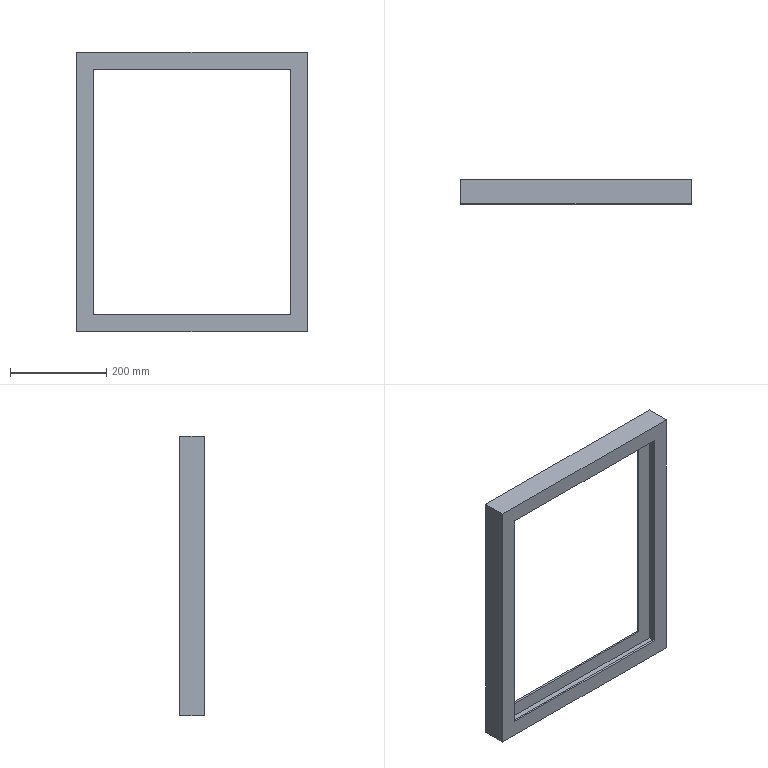Part | SolidWorks | features ICE 2, Extrusion 1 | 1 solid | 20 faces | box 480 x 50 x 580 mm | volume 907872 mm3 | plane 20
STEP:
#1=CARTESIAN_POINT('',(-10.735,12.749,35.));
#2=VERTEX_POINT('',#1);
#3=CARTESIAN_POINT('',(-10.735,8.749,35.));
#4=VERTEX_POINT('',#3);
#5=CARTESIAN_POINT('',(-10.735,8.749,35.));
#6=DIRECTION('',(0.,-1.,0.));
#7=VECTOR('',#6,1000.);
#8=LINE('',#5,#7);
#9=EDGE_CURVE('',#2,#4,#8,.T.);
#10=ORIENTED_EDGE('',*,*,#9,.F.);
#11=CARTESIAN_POINT('',(-10.735,12.749,545.));
#12=VERTEX_POINT('',#11);
#13=CARTESIAN_POINT('',(-10.735,12.749,580.));
#14=DIRECTION('',(0.,0.,-1.));
#15=VECTOR('',#14,1000.);
#16=LINE('',#13,#15);
#17=EDGE_CURVE('',#12,#2,#16,.T.);
#18=ORIENTED_EDGE('',*,*,#17,.F.);
#19=CARTESIAN_POINT('',(-10.735,8.749,545.));
#20=VERTEX_POINT('',#19);
#21=CARTESIAN_POINT('',(-10.735,8.749,545.));
#22=DIRECTION('',(0.,1.,0.));
#23=VECTOR('',#22,1000.);
#24=LINE('',#21,#23);
#25=EDGE_CURVE('',#20,#12,#24,.T.);
#26=ORIENTED_EDGE('',*,*,#25,.F.);
#27=CARTESIAN_POINT('',(-10.735,8.749,580.));
#28=DIRECTION('',(0.,0.,-1.));
#29=VECTOR('',#28,1000.);
#30=LINE('',#27,#29);
#31=EDGE_CURVE('',#20,#4,#30,.T.);
#32=ORIENTED_EDGE('',*,*,#31,.T.);
#33=EDGE_LOOP('',(#10,#18,#26,#32));
#34=FACE_OUTER_BOUND('',#33,.T.);
#35=CARTESIAN_POINT('',(-10.735,8.749,580.));
#36=DIRECTION('',(-1.,0.,0.));
#37=DIRECTION('',(0.,0.,1.));
#38=AXIS2_PLACEMENT_3D('',#35,#36,#37);
#39=PLANE('',#38);
#40=ADVANCED_FACE('',(#34),#39,.F.);
#41=CARTESIAN_POINT('',(-10.735,-33.251,35.));
#42=VERTEX_POINT('',#41);
#43=CARTESIAN_POINT('',(-10.735,-37.251,35.));
#44=VERTEX_POINT('',#43);
#45=CARTESIAN_POINT('',(-10.735,-33.251,35.));
#46=DIRECTION('',(0.,-1.,0.));
#47=VECTOR('',#46,1000.);
#48=LINE('',#45,#47);
#49=EDGE_CURVE('',#42,#44,#48,.T.);
#50=ORIENTED_EDGE('',*,*,#49,.F.);
#51=CARTESIAN_POINT('',(-10.735,-33.251,545.));
#52=VERTEX_POINT('',#51);
#53=CARTESIAN_POINT('',(-10.735,-33.251,580.));
#54=DIRECTION('',(0.,0.,-1.));
#55=VECTOR('',#54,1000.);
#56=LINE('',#53,#55);
#57=EDGE_CURVE('',#52,#42,#56,.T.);
#58=ORIENTED_EDGE('',*,*,#57,.F.);
#59=CARTESIAN_POINT('',(-10.735,-37.251,545.));
#60=VERTEX_POINT('',#59);
#61=CARTESIAN_POINT('',(-10.735,-33.251,545.));
#62=DIRECTION('',(0.,1.,0.));
#63=VECTOR('',#62,1000.);
#64=LINE('',#61,#63);
#65=EDGE_CURVE('',#60,#52,#64,.T.);
#66=ORIENTED_EDGE('',*,*,#65,.F.);
#67=CARTESIAN_POINT('',(-10.735,-37.251,580.));
#68=DIRECTION('',(0.,0.,-1.));
#69=VECTOR('',#68,1000.);
#70=LINE('',#67,#69);
#71=EDGE_CURVE('',#60,#44,#70,.T.);
#72=ORIENTED_EDGE('',*,*,#71,.T.);
#73=EDGE_LOOP('',(#50,#58,#66,#72));
#74=FACE_OUTER_BOUND('',#73,.T.);
#75=CARTESIAN_POINT('',(-10.735,-33.251,580.));
#76=DIRECTION('',(-1.,0.,0.));
#77=DIRECTION('',(0.,0.,1.));
#78=AXIS2_PLACEMENT_3D('',#75,#76,#77);
#79=PLANE('',#78);
#80=ADVANCED_FACE('',(#74),#79,.F.);
#81=CARTESIAN_POINT('',(399.265,-33.251,35.));
#82=VERTEX_POINT('',#81);
#83=CARTESIAN_POINT('',(399.265,-33.251,545.));
#84=VERTEX_POINT('',#83);
#85=CARTESIAN_POINT('',(399.265,-33.251,0.));
#86=DIRECTION('',(0.,0.,1.));
#87=VECTOR('',#86,1000.);
#88=LINE('',#85,#87);
#89=EDGE_CURVE('',#82,#84,#88,.T.);
#90=ORIENTED_EDGE('',*,*,#89,.T.);
#91=CARTESIAN_POINT('',(430.265,-33.251,545.));
#92=DIRECTION('',(-1.,0.,0.));
#93=VECTOR('',#92,1000.);
#94=LINE('',#91,#93);
#95=EDGE_CURVE('',#84,#52,#94,.T.);
#96=ORIENTED_EDGE('',*,*,#95,.T.);
#97=ORIENTED_EDGE('',*,*,#57,.T.);
#98=CARTESIAN_POINT('',(430.265,-33.251,35.));
#99=DIRECTION('',(-1.,0.,0.));
#100=VECTOR('',#99,1000.);
#101=LINE('',#98,#100);
#102=EDGE_CURVE('',#82,#42,#101,.T.);
#103=ORIENTED_EDGE('',*,*,#102,.F.);
#104=EDGE_LOOP('',(#90,#96,#97,#103));
#105=FACE_BOUND('',#104,.T.);
#106=CARTESIAN_POINT('',(-41.735,-33.251,576.));
#107=VERTEX_POINT('',#106);
#108=CARTESIAN_POINT('',(-41.735,-33.251,4.));
#109=VERTEX_POINT('',#108);
#110=CARTESIAN_POINT('',(-41.735,-33.251,580.));
#111=DIRECTION('',(0.,0.,-1.));
#112=VECTOR('',#111,1000.);
#113=LINE('',#110,#112);
#114=EDGE_CURVE('',#107,#109,#113,.T.);
#115=ORIENTED_EDGE('',*,*,#114,.F.);
#116=CARTESIAN_POINT('',(430.265,-33.251,576.));
#117=VERTEX_POINT('',#116);
#118=CARTESIAN_POINT('',(430.265,-33.251,576.));
#119=DIRECTION('',(-1.,0.,0.));
#120=VECTOR('',#119,1000.);
#121=LINE('',#118,#120);
#122=EDGE_CURVE('',#117,#107,#121,.T.);
#123=ORIENTED_EDGE('',*,*,#122,.F.);
#124=CARTESIAN_POINT('',(430.265,-33.251,4.));
#125=VERTEX_POINT('',#124);
#126=CARTESIAN_POINT('',(430.265,-33.251,576.));
#127=DIRECTION('',(0.,0.,1.));
#128=VECTOR('',#127,1000.);
#129=LINE('',#126,#128);
#130=EDGE_CURVE('',#125,#117,#129,.T.);
#131=ORIENTED_EDGE('',*,*,#130,.F.);
#132=CARTESIAN_POINT('',(430.265,-33.251,4.));
#133=DIRECTION('',(-1.,0.,0.));
#134=VECTOR('',#133,1000.);
#135=LINE('',#132,#134);
#136=EDGE_CURVE('',#125,#109,#135,.T.);
#137=ORIENTED_EDGE('',*,*,#136,.T.);
#138=EDGE_LOOP('',(#115,#123,#131,#137));
#139=FACE_OUTER_BOUND('',#138,.T.);
#140=CARTESIAN_POINT('',(-41.735,-33.251,580.));
#141=DIRECTION('',(0.,-1.,0.));
#142=DIRECTION('',(0.,0.,-1.));
#143=AXIS2_PLACEMENT_3D('',#140,#141,#142);
#144=PLANE('',#143);
#145=ADVANCED_FACE('',(#105,#139),#144,.F.);
#146=CARTESIAN_POINT('',(-41.735,8.749,4.));
#147=VERTEX_POINT('',#146);
#148=CARTESIAN_POINT('',(-41.735,8.749,4.));
#149=DIRECTION('',(0.,-1.,0.));
#150=VECTOR('',#149,1000.);
#151=LINE('',#148,#150);
#152=EDGE_CURVE('',#147,#109,#151,.T.);
#153=ORIENTED_EDGE('',*,*,#152,.F.);
#154=CARTESIAN_POINT('',(-41.735,8.749,576.));
#155=VERTEX_POINT('',#154);
#156=CARTESIAN_POINT('',(-41.735,8.749,580.));
#157=DIRECTION('',(0.,0.,-1.));
#158=VECTOR('',#157,1000.);
#159=LINE('',#156,#158);
#160=EDGE_CURVE('',#155,#147,#159,.T.);
#161=ORIENTED_EDGE('',*,*,#160,.F.);
#162=CARTESIAN_POINT('',(-41.735,8.749,576.));
#163=DIRECTION('',(0.,1.,0.));
#164=VECTOR('',#163,1000.);
#165=LINE('',#162,#164);
#166=EDGE_CURVE('',#107,#155,#165,.T.);
#167=ORIENTED_EDGE('',*,*,#166,.F.);
#168=ORIENTED_EDGE('',*,*,#114,.T.);
#169=EDGE_LOOP('',(#153,#161,#167,#168));
#170=FACE_OUTER_BOUND('',#169,.T.);
#171=CARTESIAN_POINT('',(-41.735,8.749,580.));
#172=DIRECTION('',(-1.,0.,0.));
#173=DIRECTION('',(0.,0.,1.));
#174=AXIS2_PLACEMENT_3D('',#171,#172,#173);
#175=PLANE('',#174);
#176=ADVANCED_FACE('',(#170),#175,.F.);
#177=CARTESIAN_POINT('',(399.265,8.749,35.));
#178=VERTEX_POINT('',#177);
#179=CARTESIAN_POINT('',(399.265,8.749,545.));
#180=VERTEX_POINT('',#179);
#181=CARTESIAN_POINT('',(399.265,8.749,0.));
#182=DIRECTION('',(0.,0.,1.));
#183=VECTOR('',#182,1000.);
#184=LINE('',#181,#183);
#185=EDGE_CURVE('',#178,#180,#184,.T.);
#186=ORIENTED_EDGE('',*,*,#185,.F.);
#187=CARTESIAN_POINT('',(430.265,8.749,35.));
#188=DIRECTION('',(-1.,0.,0.));
#189=VECTOR('',#188,1000.);
#190=LINE('',#187,#189);
#191=EDGE_CURVE('',#178,#4,#190,.T.);
#192=ORIENTED_EDGE('',*,*,#191,.T.);
#193=ORIENTED_EDGE('',*,*,#31,.F.);
#194=CARTESIAN_POINT('',(430.265,8.749,545.));
#195=DIRECTION('',(-1.,0.,0.));
#196=VECTOR('',#195,1000.);
#197=LINE('',#194,#196);
#198=EDGE_CURVE('',#180,#20,#197,.T.);
#199=ORIENTED_EDGE('',*,*,#198,.F.);
#200=EDGE_LOOP('',(#186,#192,#193,#199));
#201=FACE_BOUND('',#200,.T.);
#202=ORIENTED_EDGE('',*,*,#160,.T.);
#203=CARTESIAN_POINT('',(430.265,8.749,4.));
#204=VERTEX_POINT('',#203);
#205=CARTESIAN_POINT('',(-10.735,8.749,4.));
#206=DIRECTION('',(-1.,0.,0.));
#207=VECTOR('',#206,1000.);
#208=LINE('',#205,#207);
#209=EDGE_CURVE('',#204,#147,#208,.T.);
#210=ORIENTED_EDGE('',*,*,#209,.F.);
#211=CARTESIAN_POINT('',(430.265,8.749,576.));
#212=VERTEX_POINT('',#211);
#213=CARTESIAN_POINT('',(430.265,8.749,545.));
#214=DIRECTION('',(0.,0.,-1.));
#215=VECTOR('',#214,1000.);
#216=LINE('',#213,#215);
#217=EDGE_CURVE('',#212,#204,#216,.T.);
#218=ORIENTED_EDGE('',*,*,#217,.F.);
#219=CARTESIAN_POINT('',(-10.735,8.749,576.));
#220=DIRECTION('',(1.,0.,0.));
#221=VECTOR('',#220,1000.);
#222=LINE('',#219,#221);
#223=EDGE_CURVE('',#155,#212,#222,.T.);
#224=ORIENTED_EDGE('',*,*,#223,.F.);
#225=EDGE_LOOP('',(#202,#210,#218,#224));
#226=FACE_OUTER_BOUND('',#225,.T.);
#227=CARTESIAN_POINT('',(-10.735,8.749,580.));
#228=DIRECTION('',(0.,1.,0.));
#229=DIRECTION('',(0.,0.,1.));
#230=AXIS2_PLACEMENT_3D('',#227,#228,#229);
#231=PLANE('',#230);
#232=ADVANCED_FACE('',(#201,#226),#231,.F.);
#233=CARTESIAN_POINT('',(399.265,12.749,35.));
#234=VERTEX_POINT('',#233);
#235=CARTESIAN_POINT('',(399.265,12.749,545.));
#236=VERTEX_POINT('',#235);
#237=CARTESIAN_POINT('',(399.265,12.749,0.));
#238=DIRECTION('',(0.,0.,1.));
#239=VECTOR('',#238,1000.);
#240=LINE('',#237,#239);
#241=EDGE_CURVE('',#234,#236,#240,.T.);
#242=ORIENTED_EDGE('',*,*,#241,.T.);
#243=CARTESIAN_POINT('',(430.265,12.749,545.));
#244=DIRECTION('',(-1.,0.,0.));
#245=VECTOR('',#244,1000.);
#246=LINE('',#243,#245);
#247=EDGE_CURVE('',#236,#12,#246,.T.);
#248=ORIENTED_EDGE('',*,*,#247,.T.);
#249=ORIENTED_EDGE('',*,*,#17,.T.);
#250=CARTESIAN_POINT('',(430.265,12.749,35.));
#251=DIRECTION('',(-1.,0.,0.));
#252=VECTOR('',#251,1000.);
#253=LINE('',#250,#252);
#254=EDGE_CURVE('',#234,#2,#253,.T.);
#255=ORIENTED_EDGE('',*,*,#254,.F.);
#256=EDGE_LOOP('',(#242,#248,#249,#255));
#257=FACE_BOUND('',#256,.T.);
#258=CARTESIAN_POINT('',(-45.735,12.749,580.));
#259=VERTEX_POINT('',#258);
#260=CARTESIAN_POINT('',(-45.735,12.749,0.));
#261=VERTEX_POINT('',#260);
#262=CARTESIAN_POINT('',(-45.735,12.749,580.));
#263=DIRECTION('',(0.,0.,-1.));
#264=VECTOR('',#263,1000.);
#265=LINE('',#262,#264);
#266=EDGE_CURVE('',#259,#261,#265,.T.);
#267=ORIENTED_EDGE('',*,*,#266,.F.);
#268=CARTESIAN_POINT('',(434.265,12.749,580.));
#269=VERTEX_POINT('',#268);
#270=CARTESIAN_POINT('',(-10.735,12.749,580.));
#271=DIRECTION('',(-1.,0.,0.));
#272=VECTOR('',#271,1000.);
#273=LINE('',#270,#272);
#274=EDGE_CURVE('',#269,#259,#273,.T.);
#275=ORIENTED_EDGE('',*,*,#274,.F.);
#276=CARTESIAN_POINT('',(434.265,12.749,0.));
#277=VERTEX_POINT('',#276);
#278=CARTESIAN_POINT('',(434.265,12.749,0.));
#279=DIRECTION('',(0.,0.,1.));
#280=VECTOR('',#279,1000.);
#281=LINE('',#278,#280);
#282=EDGE_CURVE('',#277,#269,#281,.T.);
#283=ORIENTED_EDGE('',*,*,#282,.F.);
#284=CARTESIAN_POINT('',(-10.735,12.749,0.));
#285=DIRECTION('',(-1.,0.,0.));
#286=VECTOR('',#285,1000.);
#287=LINE('',#284,#286);
#288=EDGE_CURVE('',#277,#261,#287,.T.);
#289=ORIENTED_EDGE('',*,*,#288,.T.);
#290=EDGE_LOOP('',(#267,#275,#283,#289));
#291=FACE_OUTER_BOUND('',#290,.T.);
#292=CARTESIAN_POINT('',(-10.735,12.749,580.));
#293=DIRECTION('',(0.,-1.,0.));
#294=DIRECTION('',(1.,0.,0.));
#295=AXIS2_PLACEMENT_3D('',#292,#293,#294);
#296=PLANE('',#295);
#297=ADVANCED_FACE('',(#257,#291),#296,.F.);
#298=CARTESIAN_POINT('',(-45.735,-37.251,0.));
#299=VERTEX_POINT('',#298);
#300=CARTESIAN_POINT('',(-45.735,12.749,0.));
#301=DIRECTION('',(0.,-1.,0.));
#302=VECTOR('',#301,1000.);
#303=LINE('',#300,#302);
#304=EDGE_CURVE('',#261,#299,#303,.T.);
#305=ORIENTED_EDGE('',*,*,#304,.T.);
#306=CARTESIAN_POINT('',(-45.735,-37.251,580.));
#307=VERTEX_POINT('',#306);
#308=CARTESIAN_POINT('',(-45.735,-37.251,580.));
#309=DIRECTION('',(0.,0.,-1.));
#310=VECTOR('',#309,1000.);
#311=LINE('',#308,#310);
#312=EDGE_CURVE('',#307,#299,#311,.T.);
#313=ORIENTED_EDGE('',*,*,#312,.F.);
#314=CARTESIAN_POINT('',(-45.735,12.749,580.));
#315=DIRECTION('',(0.,-1.,0.));
#316=VECTOR('',#315,1000.);
#317=LINE('',#314,#316);
#318=EDGE_CURVE('',#259,#307,#317,.T.);
#319=ORIENTED_EDGE('',*,*,#318,.F.);
#320=ORIENTED_EDGE('',*,*,#266,.T.);
#321=EDGE_LOOP('',(#305,#313,#319,#320));
#322=FACE_OUTER_BOUND('',#321,.T.);
#323=CARTESIAN_POINT('',(-45.735,12.749,580.));
#324=DIRECTION('',(1.,0.,0.));
#325=DIRECTION('',(0.,0.,-1.));
#326=AXIS2_PLACEMENT_3D('',#323,#324,#325);
#327=PLANE('',#326);
#328=ADVANCED_FACE('',(#322),#327,.F.);
#329=CARTESIAN_POINT('',(399.265,-37.251,35.));
#330=VERTEX_POINT('',#329);
#331=CARTESIAN_POINT('',(399.265,-37.251,545.));
#332=VERTEX_POINT('',#331);
#333=CARTESIAN_POINT('',(399.265,-37.251,0.));
#334=DIRECTION('',(0.,0.,1.));
#335=VECTOR('',#334,1000.);
#336=LINE('',#333,#335);
#337=EDGE_CURVE('',#330,#332,#336,.T.);
#338=ORIENTED_EDGE('',*,*,#337,.F.);
#339=CARTESIAN_POINT('',(430.265,-37.251,35.));
#340=DIRECTION('',(-1.,0.,0.));
#341=VECTOR('',#340,1000.);
#342=LINE('',#339,#341);
#343=EDGE_CURVE('',#330,#44,#342,.T.);
#344=ORIENTED_EDGE('',*,*,#343,.T.);
#345=ORIENTED_EDGE('',*,*,#71,.F.);
#346=CARTESIAN_POINT('',(430.265,-37.251,545.));
#347=DIRECTION('',(-1.,0.,0.));
#348=VECTOR('',#347,1000.);
#349=LINE('',#346,#348);
#350=EDGE_CURVE('',#332,#60,#349,.T.);
#351=ORIENTED_EDGE('',*,*,#350,.F.);
#352=EDGE_LOOP('',(#338,#344,#345,#351));
#353=FACE_BOUND('',#352,.T.);
#354=CARTESIAN_POINT('',(434.265,-37.251,0.));
#355=VERTEX_POINT('',#354);
#356=CARTESIAN_POINT('',(-45.735,-37.251,0.));
#357=DIRECTION('',(1.,0.,0.));
#358=VECTOR('',#357,1000.);
#359=LINE('',#356,#358);
#360=EDGE_CURVE('',#299,#355,#359,.T.);
#361=ORIENTED_EDGE('',*,*,#360,.T.);
#362=CARTESIAN_POINT('',(434.265,-37.251,580.));
#363=VERTEX_POINT('',#362);
#364=CARTESIAN_POINT('',(434.265,-37.251,0.));
#365=DIRECTION('',(0.,0.,1.));
#366=VECTOR('',#365,1000.);
#367=LINE('',#364,#366);
#368=EDGE_CURVE('',#355,#363,#367,.T.);
#369=ORIENTED_EDGE('',*,*,#368,.T.);
#370=CARTESIAN_POINT('',(-45.735,-37.251,580.));
#371=DIRECTION('',(1.,0.,0.));
#372=VECTOR('',#371,1000.);
#373=LINE('',#370,#372);
#374=EDGE_CURVE('',#307,#363,#373,.T.);
#375=ORIENTED_EDGE('',*,*,#374,.F.);
#376=ORIENTED_EDGE('',*,*,#312,.T.);
#377=EDGE_LOOP('',(#361,#369,#375,#376));
#378=FACE_OUTER_BOUND('',#377,.T.);
#379=CARTESIAN_POINT('',(-45.735,-37.251,580.));
#380=DIRECTION('',(0.,1.,0.));
#381=DIRECTION('',(0.,0.,1.));
#382=AXIS2_PLACEMENT_3D('',#379,#380,#381);
#383=PLANE('',#382);
#384=ADVANCED_FACE('',(#353,#378),#383,.F.);
#385=ORIENTED_EDGE('',*,*,#374,.T.);
#386=CARTESIAN_POINT('',(434.265,12.749,580.));
#387=DIRECTION('',(0.,1.,0.));
#388=VECTOR('',#387,1000.);
#389=LINE('',#386,#388);
#390=EDGE_CURVE('',#363,#269,#389,.T.);
#391=ORIENTED_EDGE('',*,*,#390,.T.);
#392=ORIENTED_EDGE('',*,*,#274,.T.);
#393=ORIENTED_EDGE('',*,*,#318,.T.);
#394=EDGE_LOOP('',(#385,#391,#392,#393));
#395=FACE_OUTER_BOUND('',#394,.T.);
#396=CARTESIAN_POINT('',(0.,0.,580.));
#397=DIRECTION('',(0.,0.,1.));
#398=DIRECTION('',(1.,0.,0.));
#399=AXIS2_PLACEMENT_3D('',#396,#397,#398);
#400=PLANE('',#399);
#401=ADVANCED_FACE('',(#395),#400,.T.);
#402=CARTESIAN_POINT('',(434.265,12.749,0.));
#403=DIRECTION('',(0.,1.,0.));
#404=VECTOR('',#403,1000.);
#405=LINE('',#402,#404);
#406=EDGE_CURVE('',#355,#277,#405,.T.);
#407=ORIENTED_EDGE('',*,*,#406,.F.);
#408=ORIENTED_EDGE('',*,*,#360,.F.);
#409=ORIENTED_EDGE('',*,*,#304,.F.);
#410=ORIENTED_EDGE('',*,*,#288,.F.);
#411=EDGE_LOOP('',(#407,#408,#409,#410));
#412=FACE_OUTER_BOUND('',#411,.T.);
#413=CARTESIAN_POINT('',(0.,0.,0.));
#414=DIRECTION('',(0.,0.,1.));
#415=DIRECTION('',(1.,0.,0.));
#416=AXIS2_PLACEMENT_3D('',#413,#414,#415);
#417=PLANE('',#416);
#418=ADVANCED_FACE('',(#412),#417,.F.);
#419=ORIENTED_EDGE('',*,*,#95,.F.);
#420=CARTESIAN_POINT('',(399.265,-33.251,545.));
#421=DIRECTION('',(0.,-1.,0.));
#422=VECTOR('',#421,1000.);
#423=LINE('',#420,#422);
#424=EDGE_CURVE('',#84,#332,#423,.T.);
#425=ORIENTED_EDGE('',*,*,#424,.T.);
#426=ORIENTED_EDGE('',*,*,#350,.T.);
#427=ORIENTED_EDGE('',*,*,#65,.T.);
#428=EDGE_LOOP('',(#419,#425,#426,#427));
#429=FACE_OUTER_BOUND('',#428,.T.);
#430=CARTESIAN_POINT('',(430.265,-33.251,545.));
#431=DIRECTION('',(0.,0.,1.));
#432=DIRECTION('',(1.,0.,0.));
#433=AXIS2_PLACEMENT_3D('',#430,#431,#432);
#434=PLANE('',#433);
#435=ADVANCED_FACE('',(#429),#434,.F.);
#436=ORIENTED_EDGE('',*,*,#247,.F.);
#437=CARTESIAN_POINT('',(399.265,8.749,545.));
#438=DIRECTION('',(0.,-1.,0.));
#439=VECTOR('',#438,1000.);
#440=LINE('',#437,#439);
#441=EDGE_CURVE('',#236,#180,#440,.T.);
#442=ORIENTED_EDGE('',*,*,#441,.T.);
#443=ORIENTED_EDGE('',*,*,#198,.T.);
#444=ORIENTED_EDGE('',*,*,#25,.T.);
#445=EDGE_LOOP('',(#436,#442,#443,#444));
#446=FACE_OUTER_BOUND('',#445,.T.);
#447=CARTESIAN_POINT('',(430.265,8.749,545.));
#448=DIRECTION('',(0.,0.,1.));
#449=DIRECTION('',(1.,0.,0.));
#450=AXIS2_PLACEMENT_3D('',#447,#448,#449);
#451=PLANE('',#450);
#452=ADVANCED_FACE('',(#446),#451,.F.);
#453=ORIENTED_EDGE('',*,*,#166,.T.);
#454=ORIENTED_EDGE('',*,*,#223,.T.);
#455=CARTESIAN_POINT('',(430.265,8.749,576.));
#456=DIRECTION('',(0.,1.,0.));
#457=VECTOR('',#456,1000.);
#458=LINE('',#455,#457);
#459=EDGE_CURVE('',#117,#212,#458,.T.);
#460=ORIENTED_EDGE('',*,*,#459,.F.);
#461=ORIENTED_EDGE('',*,*,#122,.T.);
#462=EDGE_LOOP('',(#453,#454,#460,#461));
#463=FACE_OUTER_BOUND('',#462,.T.);
#464=CARTESIAN_POINT('',(430.265,8.749,576.));
#465=DIRECTION('',(0.,0.,1.));
#466=DIRECTION('',(1.,0.,0.));
#467=AXIS2_PLACEMENT_3D('',#464,#465,#466);
#468=PLANE('',#467);
#469=ADVANCED_FACE('',(#463),#468,.F.);
#470=ORIENTED_EDGE('',*,*,#191,.F.);
#471=CARTESIAN_POINT('',(399.265,8.749,35.));
#472=DIRECTION('',(0.,1.,0.));
#473=VECTOR('',#472,1000.);
#474=LINE('',#471,#473);
#475=EDGE_CURVE('',#178,#234,#474,.T.);
#476=ORIENTED_EDGE('',*,*,#475,.T.);
#477=ORIENTED_EDGE('',*,*,#254,.T.);
#478=ORIENTED_EDGE('',*,*,#9,.T.);
#479=EDGE_LOOP('',(#470,#476,#477,#478));
#480=FACE_OUTER_BOUND('',#479,.T.);
#481=CARTESIAN_POINT('',(430.265,8.749,35.));
#482=DIRECTION('',(0.,0.,-1.));
#483=DIRECTION('',(-1.,0.,0.));
#484=AXIS2_PLACEMENT_3D('',#481,#482,#483);
#485=PLANE('',#484);
#486=ADVANCED_FACE('',(#480),#485,.F.);
#487=ORIENTED_EDGE('',*,*,#343,.F.);
#488=CARTESIAN_POINT('',(399.265,-33.251,35.));
#489=DIRECTION('',(0.,1.,0.));
#490=VECTOR('',#489,1000.);
#491=LINE('',#488,#490);
#492=EDGE_CURVE('',#330,#82,#491,.T.);
#493=ORIENTED_EDGE('',*,*,#492,.T.);
#494=ORIENTED_EDGE('',*,*,#102,.T.);
#495=ORIENTED_EDGE('',*,*,#49,.T.);
#496=EDGE_LOOP('',(#487,#493,#494,#495));
#497=FACE_OUTER_BOUND('',#496,.T.);
#498=CARTESIAN_POINT('',(430.265,-33.251,35.));
#499=DIRECTION('',(0.,0.,-1.));
#500=DIRECTION('',(-1.,0.,0.));
#501=AXIS2_PLACEMENT_3D('',#498,#499,#500);
#502=PLANE('',#501);
#503=ADVANCED_FACE('',(#497),#502,.F.);
#504=ORIENTED_EDGE('',*,*,#152,.T.);
#505=ORIENTED_EDGE('',*,*,#136,.F.);
#506=CARTESIAN_POINT('',(430.265,8.749,4.));
#507=DIRECTION('',(0.,-1.,0.));
#508=VECTOR('',#507,1000.);
#509=LINE('',#506,#508);
#510=EDGE_CURVE('',#204,#125,#509,.T.);
#511=ORIENTED_EDGE('',*,*,#510,.F.);
#512=ORIENTED_EDGE('',*,*,#209,.T.);
#513=EDGE_LOOP('',(#504,#505,#511,#512));
#514=FACE_OUTER_BOUND('',#513,.T.);
#515=CARTESIAN_POINT('',(430.265,8.749,4.));
#516=DIRECTION('',(0.,0.,-1.));
#517=DIRECTION('',(-1.,0.,0.));
#518=AXIS2_PLACEMENT_3D('',#515,#516,#517);
#519=PLANE('',#518);
#520=ADVANCED_FACE('',(#514),#519,.F.);
#521=ORIENTED_EDGE('',*,*,#441,.F.);
#522=ORIENTED_EDGE('',*,*,#241,.F.);
#523=ORIENTED_EDGE('',*,*,#475,.F.);
#524=ORIENTED_EDGE('',*,*,#185,.T.);
#525=EDGE_LOOP('',(#521,#522,#523,#524));
#526=FACE_OUTER_BOUND('',#525,.T.);
#527=CARTESIAN_POINT('',(399.265,8.749,0.));
#528=DIRECTION('',(-1.,0.,0.));
#529=DIRECTION('',(0.,0.,1.));
#530=AXIS2_PLACEMENT_3D('',#527,#528,#529);
#531=PLANE('',#530);
#532=ADVANCED_FACE('',(#526),#531,.T.);
#533=ORIENTED_EDGE('',*,*,#424,.F.);
#534=ORIENTED_EDGE('',*,*,#89,.F.);
#535=ORIENTED_EDGE('',*,*,#492,.F.);
#536=ORIENTED_EDGE('',*,*,#337,.T.);
#537=EDGE_LOOP('',(#533,#534,#535,#536));
#538=FACE_OUTER_BOUND('',#537,.T.);
#539=CARTESIAN_POINT('',(399.265,-33.251,0.));
#540=DIRECTION('',(-1.,0.,0.));
#541=DIRECTION('',(0.,0.,1.));
#542=AXIS2_PLACEMENT_3D('',#539,#540,#541);
#543=PLANE('',#542);
#544=ADVANCED_FACE('',(#538),#543,.T.);
#545=ORIENTED_EDGE('',*,*,#459,.T.);
#546=ORIENTED_EDGE('',*,*,#217,.T.);
#547=ORIENTED_EDGE('',*,*,#510,.T.);
#548=ORIENTED_EDGE('',*,*,#130,.T.);
#549=EDGE_LOOP('',(#545,#546,#547,#548));
#550=FACE_OUTER_BOUND('',#549,.T.);
#551=CARTESIAN_POINT('',(430.265,8.749,0.));
#552=DIRECTION('',(-1.,0.,0.));
#553=DIRECTION('',(0.,0.,1.));
#554=AXIS2_PLACEMENT_3D('',#551,#552,#553);
#555=PLANE('',#554);
#556=ADVANCED_FACE('',(#550),#555,.T.);
#557=ORIENTED_EDGE('',*,*,#390,.F.);
#558=ORIENTED_EDGE('',*,*,#368,.F.);
#559=ORIENTED_EDGE('',*,*,#406,.T.);
#560=ORIENTED_EDGE('',*,*,#282,.T.);
#561=EDGE_LOOP('',(#557,#558,#559,#560));
#562=FACE_OUTER_BOUND('',#561,.T.);
#563=CARTESIAN_POINT('',(434.265,12.749,0.));
#564=DIRECTION('',(1.,0.,0.));
#565=DIRECTION('',(0.,0.,-1.));
#566=AXIS2_PLACEMENT_3D('',#563,#564,#565);
#567=PLANE('',#566);
#568=ADVANCED_FACE('',(#562),#567,.T.);
#569=CLOSED_SHELL('',(#40,#80,#145,#176,#232,#297,#328,#384,#401,#418,#435,#452,#469,#486,#503,#520,#532,#544,#556,#568));
#570=MANIFOLD_SOLID_BREP('',#569);
#571=CARTESIAN_POINT('',(0.,0.,0.));
#572=DIRECTION('',(0.,0.,1.));
#573=DIRECTION('',(1.,0.,0.));
#574=AXIS2_PLACEMENT_3D('',#571,#572,#573);
#575=(LENGTH_UNIT()NAMED_UNIT(*)SI_UNIT(.MILLI.,.METRE.));
#576=UNCERTAINTY_MEASURE_WITH_UNIT(LENGTH_MEASURE(0.00001),#575,'','');
#577=(NAMED_UNIT(*)PLANE_ANGLE_UNIT()SI_UNIT($,.RADIAN.));
#578=(NAMED_UNIT(*)SI_UNIT($,.STERADIAN.)SOLID_ANGLE_UNIT());
#579=(GEOMETRIC_REPRESENTATION_CONTEXT(3)GLOBAL_UNCERTAINTY_ASSIGNED_CONTEXT((#576))GLOBAL_UNIT_ASSIGNED_CONTEXT((#575,#577,#578))REPRESENTATION_CONTEXT('',''));
#580=ADVANCED_BREP_SHAPE_REPRESENTATION('',(#570,#574),#579);